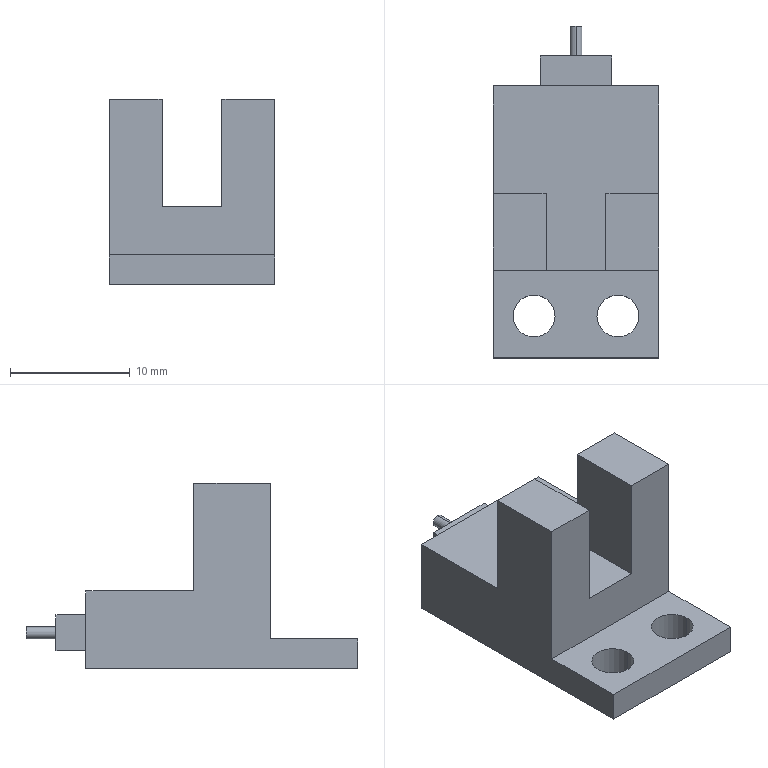Part | SolidWorks | features BaseBody 1 | 1 solid | 26 faces | box 13.8 x 27.7 x 15.5 mm | volume 2139 mm3 | plane 20 | cylinder 6 | commonest cylinder face diameters 3.5 x4 1 x2
STEP:
#1=CARTESIAN_POINT('',(5.25,-14.7,0.));
#2=VERTEX_POINT('',#1);
#3=CARTESIAN_POINT('',(1.75,-14.7,0.));
#4=VERTEX_POINT('',#3);
#5=CARTESIAN_POINT('',(3.5,-14.7,0.));
#6=DIRECTION('',(0.,0.,-1.));
#7=DIRECTION('',(1.,0.,0.));
#8=AXIS2_PLACEMENT_3D('',#5,#6,#7);
#9=CIRCLE('',#8,1.75);
#10=EDGE_CURVE('',#2,#4,#9,.T.);
#11=ORIENTED_EDGE('',*,*,#10,.T.);
#12=CARTESIAN_POINT('',(1.75,-14.7,2.5));
#13=VERTEX_POINT('',#12);
#14=CARTESIAN_POINT('',(1.75,-14.7,2.5));
#15=DIRECTION('',(0.,0.,1.));
#16=VECTOR('',#15,1000.);
#17=LINE('',#14,#16);
#18=EDGE_CURVE('',#4,#13,#17,.T.);
#19=ORIENTED_EDGE('',*,*,#18,.T.);
#20=CARTESIAN_POINT('',(5.25,-14.7,2.5));
#21=VERTEX_POINT('',#20);
#22=CARTESIAN_POINT('',(3.5,-14.7,2.5));
#23=DIRECTION('',(0.,0.,-1.));
#24=DIRECTION('',(1.,0.,0.));
#25=AXIS2_PLACEMENT_3D('',#22,#23,#24);
#26=CIRCLE('',#25,1.75);
#27=EDGE_CURVE('',#21,#13,#26,.T.);
#28=ORIENTED_EDGE('',*,*,#27,.F.);
#29=CARTESIAN_POINT('',(5.25,-14.7,2.5));
#30=DIRECTION('',(0.,0.,1.));
#31=VECTOR('',#30,1000.);
#32=LINE('',#29,#31);
#33=EDGE_CURVE('',#2,#21,#32,.T.);
#34=ORIENTED_EDGE('',*,*,#33,.F.);
#35=EDGE_LOOP('',(#11,#19,#28,#34));
#36=FACE_OUTER_BOUND('',#35,.T.);
#37=CARTESIAN_POINT('',(3.5,-14.7,2.5));
#38=DIRECTION('',(0.,0.,1.));
#39=DIRECTION('',(1.,0.,0.));
#40=AXIS2_PLACEMENT_3D('',#37,#38,#39);
#41=CYLINDRICAL_SURFACE('',#40,1.75);
#42=ADVANCED_FACE('',(#36),#41,.F.);
#43=CARTESIAN_POINT('',(-1.75,-14.7,0.));
#44=VERTEX_POINT('',#43);
#45=CARTESIAN_POINT('',(-5.25,-14.7,0.));
#46=VERTEX_POINT('',#45);
#47=CARTESIAN_POINT('',(-3.5,-14.7,0.));
#48=DIRECTION('',(0.,0.,-1.));
#49=DIRECTION('',(1.,0.,0.));
#50=AXIS2_PLACEMENT_3D('',#47,#48,#49);
#51=CIRCLE('',#50,1.75);
#52=EDGE_CURVE('',#44,#46,#51,.T.);
#53=ORIENTED_EDGE('',*,*,#52,.T.);
#54=CARTESIAN_POINT('',(-5.25,-14.7,2.5));
#55=VERTEX_POINT('',#54);
#56=CARTESIAN_POINT('',(-5.25,-14.7,2.5));
#57=DIRECTION('',(0.,0.,1.));
#58=VECTOR('',#57,1000.);
#59=LINE('',#56,#58);
#60=EDGE_CURVE('',#46,#55,#59,.T.);
#61=ORIENTED_EDGE('',*,*,#60,.T.);
#62=CARTESIAN_POINT('',(-1.75,-14.7,2.5));
#63=VERTEX_POINT('',#62);
#64=CARTESIAN_POINT('',(-3.5,-14.7,2.5));
#65=DIRECTION('',(0.,0.,-1.));
#66=DIRECTION('',(1.,0.,0.));
#67=AXIS2_PLACEMENT_3D('',#64,#65,#66);
#68=CIRCLE('',#67,1.75);
#69=EDGE_CURVE('',#63,#55,#68,.T.);
#70=ORIENTED_EDGE('',*,*,#69,.F.);
#71=CARTESIAN_POINT('',(-1.75,-14.7,2.5));
#72=DIRECTION('',(0.,0.,1.));
#73=VECTOR('',#72,1000.);
#74=LINE('',#71,#73);
#75=EDGE_CURVE('',#44,#63,#74,.T.);
#76=ORIENTED_EDGE('',*,*,#75,.F.);
#77=EDGE_LOOP('',(#53,#61,#70,#76));
#78=FACE_OUTER_BOUND('',#77,.T.);
#79=CARTESIAN_POINT('',(-3.5,-14.7,2.5));
#80=DIRECTION('',(0.,0.,1.));
#81=DIRECTION('',(1.,0.,0.));
#82=AXIS2_PLACEMENT_3D('',#79,#80,#81);
#83=CYLINDRICAL_SURFACE('',#82,1.75);
#84=ADVANCED_FACE('',(#78),#83,.F.);
#85=CARTESIAN_POINT('',(0.,9.5,2.5));
#86=VERTEX_POINT('',#85);
#87=CARTESIAN_POINT('',(0.,9.5,3.5));
#88=VERTEX_POINT('',#87);
#89=CARTESIAN_POINT('',(0.,9.5,3.));
#90=DIRECTION('',(0.,-1.,0.));
#91=DIRECTION('',(0.,0.,-1.));
#92=AXIS2_PLACEMENT_3D('',#89,#90,#91);
#93=CIRCLE('',#92,0.5);
#94=EDGE_CURVE('',#86,#88,#93,.T.);
#95=ORIENTED_EDGE('',*,*,#94,.T.);
#96=CARTESIAN_POINT('',(0.,7.,3.5));
#97=VERTEX_POINT('',#96);
#98=CARTESIAN_POINT('',(0.,9.5,3.5));
#99=DIRECTION('',(0.,-1.,0.));
#100=VECTOR('',#99,1000.);
#101=LINE('',#98,#100);
#102=EDGE_CURVE('',#88,#97,#101,.T.);
#103=ORIENTED_EDGE('',*,*,#102,.T.);
#104=CARTESIAN_POINT('',(0.,7.,2.5));
#105=VERTEX_POINT('',#104);
#106=CARTESIAN_POINT('',(0.,7.,3.));
#107=DIRECTION('',(0.,-1.,0.));
#108=DIRECTION('',(0.,0.,-1.));
#109=AXIS2_PLACEMENT_3D('',#106,#107,#108);
#110=CIRCLE('',#109,0.5);
#111=EDGE_CURVE('',#105,#97,#110,.T.);
#112=ORIENTED_EDGE('',*,*,#111,.F.);
#113=CARTESIAN_POINT('',(0.,9.5,2.5));
#114=DIRECTION('',(0.,-1.,0.));
#115=VECTOR('',#114,1000.);
#116=LINE('',#113,#115);
#117=EDGE_CURVE('',#86,#105,#116,.T.);
#118=ORIENTED_EDGE('',*,*,#117,.F.);
#119=EDGE_LOOP('',(#95,#103,#112,#118));
#120=FACE_OUTER_BOUND('',#119,.T.);
#121=CARTESIAN_POINT('',(0.,9.5,3.));
#122=DIRECTION('',(0.,-1.,0.));
#123=DIRECTION('',(0.,0.,-1.));
#124=AXIS2_PLACEMENT_3D('',#121,#122,#123);
#125=CYLINDRICAL_SURFACE('',#124,0.5);
#126=ADVANCED_FACE('',(#120),#125,.T.);
#127=CARTESIAN_POINT('',(-6.9,-18.2,0.));
#128=VERTEX_POINT('',#127);
#129=CARTESIAN_POINT('',(6.9,-18.2,0.));
#130=VERTEX_POINT('',#129);
#131=CARTESIAN_POINT('',(0.,-18.2,0.));
#132=DIRECTION('',(1.,0.,0.));
#133=VECTOR('',#132,1000.);
#134=LINE('',#131,#133);
#135=EDGE_CURVE('',#128,#130,#134,.T.);
#136=ORIENTED_EDGE('',*,*,#135,.F.);
#137=CARTESIAN_POINT('',(-6.9,4.5,0.));
#138=VERTEX_POINT('',#137);
#139=CARTESIAN_POINT('',(-6.9,0.,0.));
#140=DIRECTION('',(0.,-1.,0.));
#141=VECTOR('',#140,1000.);
#142=LINE('',#139,#141);
#143=EDGE_CURVE('',#138,#128,#142,.T.);
#144=ORIENTED_EDGE('',*,*,#143,.F.);
#145=CARTESIAN_POINT('',(6.9,4.5,0.));
#146=VERTEX_POINT('',#145);
#147=CARTESIAN_POINT('',(0.,4.5,0.));
#148=DIRECTION('',(-1.,0.,0.));
#149=VECTOR('',#148,1000.);
#150=LINE('',#147,#149);
#151=EDGE_CURVE('',#146,#138,#150,.T.);
#152=ORIENTED_EDGE('',*,*,#151,.F.);
#153=CARTESIAN_POINT('',(6.9,0.,0.));
#154=DIRECTION('',(0.,1.,0.));
#155=VECTOR('',#154,1000.);
#156=LINE('',#153,#155);
#157=EDGE_CURVE('',#130,#146,#156,.T.);
#158=ORIENTED_EDGE('',*,*,#157,.F.);
#159=EDGE_LOOP('',(#136,#144,#152,#158));
#160=FACE_OUTER_BOUND('',#159,.T.);
#161=ORIENTED_EDGE('',*,*,#10,.F.);
#162=CARTESIAN_POINT('',(3.5,-14.7,0.));
#163=DIRECTION('',(0.,0.,-1.));
#164=DIRECTION('',(1.,0.,0.));
#165=AXIS2_PLACEMENT_3D('',#162,#163,#164);
#166=CIRCLE('',#165,1.75);
#167=EDGE_CURVE('',#4,#2,#166,.T.);
#168=ORIENTED_EDGE('',*,*,#167,.F.);
#169=EDGE_LOOP('',(#161,#168));
#170=FACE_BOUND('',#169,.T.);
#171=ORIENTED_EDGE('',*,*,#52,.F.);
#172=CARTESIAN_POINT('',(-3.5,-14.7,0.));
#173=DIRECTION('',(0.,0.,-1.));
#174=DIRECTION('',(1.,0.,0.));
#175=AXIS2_PLACEMENT_3D('',#172,#173,#174);
#176=CIRCLE('',#175,1.75);
#177=EDGE_CURVE('',#46,#44,#176,.T.);
#178=ORIENTED_EDGE('',*,*,#177,.F.);
#179=EDGE_LOOP('',(#171,#178));
#180=FACE_BOUND('',#179,.T.);
#181=CARTESIAN_POINT('',(0.,0.,0.));
#182=DIRECTION('',(0.,0.,1.));
#183=DIRECTION('',(1.,0.,0.));
#184=AXIS2_PLACEMENT_3D('',#181,#182,#183);
#185=PLANE('',#184);
#186=ADVANCED_FACE('',(#160,#170,#180),#185,.F.);
#187=CARTESIAN_POINT('',(6.9,4.5,6.5));
#188=VERTEX_POINT('',#187);
#189=CARTESIAN_POINT('',(6.9,4.5,6.5));
#190=DIRECTION('',(0.,0.,-1.));
#191=VECTOR('',#190,1000.);
#192=LINE('',#189,#191);
#193=EDGE_CURVE('',#188,#146,#192,.T.);
#194=ORIENTED_EDGE('',*,*,#193,.F.);
#195=CARTESIAN_POINT('',(6.9,-4.5,6.5));
#196=VERTEX_POINT('',#195);
#197=CARTESIAN_POINT('',(6.9,4.5,6.5));
#198=DIRECTION('',(0.,1.,0.));
#199=VECTOR('',#198,1000.);
#200=LINE('',#197,#199);
#201=EDGE_CURVE('',#196,#188,#200,.T.);
#202=ORIENTED_EDGE('',*,*,#201,.F.);
#203=CARTESIAN_POINT('',(6.9,-4.5,15.5));
#204=VERTEX_POINT('',#203);
#205=CARTESIAN_POINT('',(6.9,-4.5,6.5));
#206=DIRECTION('',(0.,0.,-1.));
#207=VECTOR('',#206,1000.);
#208=LINE('',#205,#207);
#209=EDGE_CURVE('',#204,#196,#208,.T.);
#210=ORIENTED_EDGE('',*,*,#209,.F.);
#211=CARTESIAN_POINT('',(6.9,-10.9,15.5));
#212=VERTEX_POINT('',#211);
#213=CARTESIAN_POINT('',(6.9,4.5,15.5));
#214=DIRECTION('',(0.,1.,0.));
#215=VECTOR('',#214,1000.);
#216=LINE('',#213,#215);
#217=EDGE_CURVE('',#212,#204,#216,.T.);
#218=ORIENTED_EDGE('',*,*,#217,.F.);
#219=CARTESIAN_POINT('',(6.9,-10.9,2.5));
#220=VERTEX_POINT('',#219);
#221=CARTESIAN_POINT('',(6.9,-10.9,6.5));
#222=DIRECTION('',(0.,0.,1.));
#223=VECTOR('',#222,1000.);
#224=LINE('',#221,#223);
#225=EDGE_CURVE('',#220,#212,#224,.T.);
#226=ORIENTED_EDGE('',*,*,#225,.F.);
#227=CARTESIAN_POINT('',(6.9,-18.2,2.5));
#228=VERTEX_POINT('',#227);
#229=CARTESIAN_POINT('',(6.9,4.5,2.5));
#230=DIRECTION('',(0.,1.,0.));
#231=VECTOR('',#230,1000.);
#232=LINE('',#229,#231);
#233=EDGE_CURVE('',#228,#220,#232,.T.);
#234=ORIENTED_EDGE('',*,*,#233,.F.);
#235=CARTESIAN_POINT('',(6.9,-18.2,6.5));
#236=DIRECTION('',(0.,0.,1.));
#237=VECTOR('',#236,1000.);
#238=LINE('',#235,#237);
#239=EDGE_CURVE('',#130,#228,#238,.T.);
#240=ORIENTED_EDGE('',*,*,#239,.F.);
#241=ORIENTED_EDGE('',*,*,#157,.T.);
#242=EDGE_LOOP('',(#194,#202,#210,#218,#226,#234,#240,#241));
#243=FACE_OUTER_BOUND('',#242,.T.);
#244=CARTESIAN_POINT('',(6.9,4.5,6.5));
#245=DIRECTION('',(-1.,0.,0.));
#246=DIRECTION('',(0.,-1.,0.));
#247=AXIS2_PLACEMENT_3D('',#244,#245,#246);
#248=PLANE('',#247);
#249=ADVANCED_FACE('',(#243),#248,.F.);
#250=ORIENTED_EDGE('',*,*,#135,.T.);
#251=ORIENTED_EDGE('',*,*,#239,.T.);
#252=CARTESIAN_POINT('',(-6.9,-18.2,2.5));
#253=VERTEX_POINT('',#252);
#254=CARTESIAN_POINT('',(0.,-18.2,2.5));
#255=DIRECTION('',(1.,0.,0.));
#256=VECTOR('',#255,1000.);
#257=LINE('',#254,#256);
#258=EDGE_CURVE('',#253,#228,#257,.T.);
#259=ORIENTED_EDGE('',*,*,#258,.F.);
#260=CARTESIAN_POINT('',(-6.9,-18.2,0.));
#261=DIRECTION('',(0.,0.,1.));
#262=VECTOR('',#261,1000.);
#263=LINE('',#260,#262);
#264=EDGE_CURVE('',#128,#253,#263,.T.);
#265=ORIENTED_EDGE('',*,*,#264,.F.);
#266=EDGE_LOOP('',(#250,#251,#259,#265));
#267=FACE_OUTER_BOUND('',#266,.T.);
#268=CARTESIAN_POINT('',(0.,-18.2,0.));
#269=DIRECTION('',(0.,1.,0.));
#270=DIRECTION('',(0.,0.,1.));
#271=AXIS2_PLACEMENT_3D('',#268,#269,#270);
#272=PLANE('',#271);
#273=ADVANCED_FACE('',(#267),#272,.F.);
#274=ORIENTED_EDGE('',*,*,#264,.T.);
#275=CARTESIAN_POINT('',(-6.9,-10.9,2.5));
#276=VERTEX_POINT('',#275);
#277=CARTESIAN_POINT('',(-6.9,4.5,2.5));
#278=DIRECTION('',(0.,-1.,0.));
#279=VECTOR('',#278,1000.);
#280=LINE('',#277,#279);
#281=EDGE_CURVE('',#276,#253,#280,.T.);
#282=ORIENTED_EDGE('',*,*,#281,.F.);
#283=CARTESIAN_POINT('',(-6.9,-10.9,15.5));
#284=VERTEX_POINT('',#283);
#285=CARTESIAN_POINT('',(-6.9,-10.9,6.5));
#286=DIRECTION('',(0.,0.,-1.));
#287=VECTOR('',#286,1000.);
#288=LINE('',#285,#287);
#289=EDGE_CURVE('',#284,#276,#288,.T.);
#290=ORIENTED_EDGE('',*,*,#289,.F.);
#291=CARTESIAN_POINT('',(-6.9,-4.5,15.5));
#292=VERTEX_POINT('',#291);
#293=CARTESIAN_POINT('',(-6.9,4.5,15.5));
#294=DIRECTION('',(0.,-1.,0.));
#295=VECTOR('',#294,1000.);
#296=LINE('',#293,#295);
#297=EDGE_CURVE('',#292,#284,#296,.T.);
#298=ORIENTED_EDGE('',*,*,#297,.F.);
#299=CARTESIAN_POINT('',(-6.9,-4.5,6.5));
#300=VERTEX_POINT('',#299);
#301=CARTESIAN_POINT('',(-6.9,-4.5,6.5));
#302=DIRECTION('',(0.,0.,1.));
#303=VECTOR('',#302,1000.);
#304=LINE('',#301,#303);
#305=EDGE_CURVE('',#300,#292,#304,.T.);
#306=ORIENTED_EDGE('',*,*,#305,.F.);
#307=CARTESIAN_POINT('',(-6.9,4.5,6.5));
#308=VERTEX_POINT('',#307);
#309=CARTESIAN_POINT('',(-6.9,4.5,6.5));
#310=DIRECTION('',(0.,-1.,0.));
#311=VECTOR('',#310,1000.);
#312=LINE('',#309,#311);
#313=EDGE_CURVE('',#308,#300,#312,.T.);
#314=ORIENTED_EDGE('',*,*,#313,.F.);
#315=CARTESIAN_POINT('',(-6.9,4.5,6.5));
#316=DIRECTION('',(0.,0.,1.));
#317=VECTOR('',#316,1000.);
#318=LINE('',#315,#317);
#319=EDGE_CURVE('',#138,#308,#318,.T.);
#320=ORIENTED_EDGE('',*,*,#319,.F.);
#321=ORIENTED_EDGE('',*,*,#143,.T.);
#322=EDGE_LOOP('',(#274,#282,#290,#298,#306,#314,#320,#321));
#323=FACE_OUTER_BOUND('',#322,.T.);
#324=CARTESIAN_POINT('',(-6.9,4.5,6.5));
#325=DIRECTION('',(1.,0.,0.));
#326=DIRECTION('',(0.,1.,0.));
#327=AXIS2_PLACEMENT_3D('',#324,#325,#326);
#328=PLANE('',#327);
#329=ADVANCED_FACE('',(#323),#328,.F.);
#330=CARTESIAN_POINT('',(3.,4.5,1.5));
#331=VERTEX_POINT('',#330);
#332=CARTESIAN_POINT('',(-3.,4.5,1.5));
#333=VERTEX_POINT('',#332);
#334=CARTESIAN_POINT('',(-6.9,4.5,1.5));
#335=DIRECTION('',(-1.,0.,0.));
#336=VECTOR('',#335,1000.);
#337=LINE('',#334,#336);
#338=EDGE_CURVE('',#331,#333,#337,.T.);
#339=ORIENTED_EDGE('',*,*,#338,.F.);
#340=CARTESIAN_POINT('',(3.,4.5,4.5));
#341=VERTEX_POINT('',#340);
#342=CARTESIAN_POINT('',(3.,4.5,6.5));
#343=DIRECTION('',(0.,0.,-1.));
#344=VECTOR('',#343,1000.);
#345=LINE('',#342,#344);
#346=EDGE_CURVE('',#341,#331,#345,.T.);
#347=ORIENTED_EDGE('',*,*,#346,.F.);
#348=CARTESIAN_POINT('',(-3.,4.5,4.5));
#349=VERTEX_POINT('',#348);
#350=CARTESIAN_POINT('',(-6.9,4.5,4.5));
#351=DIRECTION('',(1.,0.,0.));
#352=VECTOR('',#351,1000.);
#353=LINE('',#350,#352);
#354=EDGE_CURVE('',#349,#341,#353,.T.);
#355=ORIENTED_EDGE('',*,*,#354,.F.);
#356=CARTESIAN_POINT('',(-3.,4.5,6.5));
#357=DIRECTION('',(0.,0.,1.));
#358=VECTOR('',#357,1000.);
#359=LINE('',#356,#358);
#360=EDGE_CURVE('',#333,#349,#359,.T.);
#361=ORIENTED_EDGE('',*,*,#360,.F.);
#362=EDGE_LOOP('',(#339,#347,#355,#361));
#363=FACE_BOUND('',#362,.T.);
#364=ORIENTED_EDGE('',*,*,#319,.T.);
#365=CARTESIAN_POINT('',(-6.9,4.5,6.5));
#366=DIRECTION('',(-1.,0.,0.));
#367=VECTOR('',#366,1000.);
#368=LINE('',#365,#367);
#369=EDGE_CURVE('',#188,#308,#368,.T.);
#370=ORIENTED_EDGE('',*,*,#369,.F.);
#371=ORIENTED_EDGE('',*,*,#193,.T.);
#372=ORIENTED_EDGE('',*,*,#151,.T.);
#373=EDGE_LOOP('',(#364,#370,#371,#372));
#374=FACE_OUTER_BOUND('',#373,.T.);
#375=CARTESIAN_POINT('',(-6.9,4.5,6.5));
#376=DIRECTION('',(0.,-1.,0.));
#377=DIRECTION('',(0.,0.,-1.));
#378=AXIS2_PLACEMENT_3D('',#375,#376,#377);
#379=PLANE('',#378);
#380=ADVANCED_FACE('',(#363,#374),#379,.F.);
#381=ORIENTED_EDGE('',*,*,#18,.F.);
#382=ORIENTED_EDGE('',*,*,#167,.T.);
#383=ORIENTED_EDGE('',*,*,#33,.T.);
#384=CARTESIAN_POINT('',(3.5,-14.7,2.5));
#385=DIRECTION('',(0.,0.,-1.));
#386=DIRECTION('',(1.,0.,0.));
#387=AXIS2_PLACEMENT_3D('',#384,#385,#386);
#388=CIRCLE('',#387,1.75);
#389=EDGE_CURVE('',#13,#21,#388,.T.);
#390=ORIENTED_EDGE('',*,*,#389,.F.);
#391=EDGE_LOOP('',(#381,#382,#383,#390));
#392=FACE_OUTER_BOUND('',#391,.T.);
#393=CARTESIAN_POINT('',(3.5,-14.7,2.5));
#394=DIRECTION('',(0.,0.,1.));
#395=DIRECTION('',(1.,0.,0.));
#396=AXIS2_PLACEMENT_3D('',#393,#394,#395);
#397=CYLINDRICAL_SURFACE('',#396,1.75);
#398=ADVANCED_FACE('',(#392),#397,.F.);
#399=ORIENTED_EDGE('',*,*,#60,.F.);
#400=ORIENTED_EDGE('',*,*,#177,.T.);
#401=ORIENTED_EDGE('',*,*,#75,.T.);
#402=CARTESIAN_POINT('',(-3.5,-14.7,2.5));
#403=DIRECTION('',(0.,0.,-1.));
#404=DIRECTION('',(1.,0.,0.));
#405=AXIS2_PLACEMENT_3D('',#402,#403,#404);
#406=CIRCLE('',#405,1.75);
#407=EDGE_CURVE('',#55,#63,#406,.T.);
#408=ORIENTED_EDGE('',*,*,#407,.F.);
#409=EDGE_LOOP('',(#399,#400,#401,#408));
#410=FACE_OUTER_BOUND('',#409,.T.);
#411=CARTESIAN_POINT('',(-3.5,-14.7,2.5));
#412=DIRECTION('',(0.,0.,1.));
#413=DIRECTION('',(1.,0.,0.));
#414=AXIS2_PLACEMENT_3D('',#411,#412,#413);
#415=CYLINDRICAL_SURFACE('',#414,1.75);
#416=ADVANCED_FACE('',(#410),#415,.F.);
#417=ORIENTED_EDGE('',*,*,#369,.T.);
#418=ORIENTED_EDGE('',*,*,#313,.T.);
#419=CARTESIAN_POINT('',(-2.5,-4.5,6.5));
#420=VERTEX_POINT('',#419);
#421=CARTESIAN_POINT('',(0.,-4.5,6.5));
#422=DIRECTION('',(1.,0.,0.));
#423=VECTOR('',#422,1000.);
#424=LINE('',#421,#423);
#425=EDGE_CURVE('',#300,#420,#424,.T.);
#426=ORIENTED_EDGE('',*,*,#425,.T.);
#427=CARTESIAN_POINT('',(-2.5,-10.9,6.5));
#428=VERTEX_POINT('',#427);
#429=CARTESIAN_POINT('',(-2.5,0.,6.5));
#430=DIRECTION('',(0.,-1.,0.));
#431=VECTOR('',#430,1000.);
#432=LINE('',#429,#431);
#433=EDGE_CURVE('',#420,#428,#432,.T.);
#434=ORIENTED_EDGE('',*,*,#433,.T.);
#435=CARTESIAN_POINT('',(2.5,-10.9,6.5));
#436=VERTEX_POINT('',#435);
#437=CARTESIAN_POINT('',(0.,-10.9,6.5));
#438=DIRECTION('',(1.,0.,0.));
#439=VECTOR('',#438,1000.);
#440=LINE('',#437,#439);
#441=EDGE_CURVE('',#428,#436,#440,.T.);
#442=ORIENTED_EDGE('',*,*,#441,.T.);
#443=CARTESIAN_POINT('',(2.5,-4.5,6.5));
#444=VERTEX_POINT('',#443);
#445=CARTESIAN_POINT('',(2.5,0.,6.5));
#446=DIRECTION('',(0.,1.,0.));
#447=VECTOR('',#446,1000.);
#448=LINE('',#445,#447);
#449=EDGE_CURVE('',#436,#444,#448,.T.);
#450=ORIENTED_EDGE('',*,*,#449,.T.);
#451=CARTESIAN_POINT('',(0.,-4.5,6.5));
#452=DIRECTION('',(1.,0.,0.));
#453=VECTOR('',#452,1000.);
#454=LINE('',#451,#453);
#455=EDGE_CURVE('',#444,#196,#454,.T.);
#456=ORIENTED_EDGE('',*,*,#455,.T.);
#457=ORIENTED_EDGE('',*,*,#201,.T.);
#458=EDGE_LOOP('',(#417,#418,#426,#434,#442,#450,#456,#457));
#459=FACE_OUTER_BOUND('',#458,.T.);
#460=CARTESIAN_POINT('',(0.,0.,6.5));
#461=DIRECTION('',(0.,0.,1.));
#462=DIRECTION('',(1.,0.,0.));
#463=AXIS2_PLACEMENT_3D('',#460,#461,#462);
#464=PLANE('',#463);
#465=ADVANCED_FACE('',(#459),#464,.T.);
#466=CARTESIAN_POINT('',(2.5,-4.5,15.5));
#467=VERTEX_POINT('',#466);
#468=CARTESIAN_POINT('',(2.5,-4.5,0.));
#469=DIRECTION('',(0.,0.,-1.));
#470=VECTOR('',#469,1000.);
#471=LINE('',#468,#470);
#472=EDGE_CURVE('',#467,#444,#471,.T.);
#473=ORIENTED_EDGE('',*,*,#472,.F.);
#474=CARTESIAN_POINT('',(0.,-4.5,15.5));
#475=DIRECTION('',(-1.,0.,0.));
#476=VECTOR('',#475,1000.);
#477=LINE('',#474,#476);
#478=EDGE_CURVE('',#204,#467,#477,.T.);
#479=ORIENTED_EDGE('',*,*,#478,.F.);
#480=ORIENTED_EDGE('',*,*,#209,.T.);
#481=ORIENTED_EDGE('',*,*,#455,.F.);
#482=EDGE_LOOP('',(#473,#479,#480,#481));
#483=FACE_OUTER_BOUND('',#482,.T.);
#484=CARTESIAN_POINT('',(0.,-4.5,0.));
#485=DIRECTION('',(0.,-1.,0.));
#486=DIRECTION('',(0.,0.,-1.));
#487=AXIS2_PLACEMENT_3D('',#484,#485,#486);
#488=PLANE('',#487);
#489=ADVANCED_FACE('',(#483),#488,.F.);
#490=CARTESIAN_POINT('',(2.5,-10.9,15.5));
#491=VERTEX_POINT('',#490);
#492=CARTESIAN_POINT('',(2.5,-10.9,15.5));
#493=DIRECTION('',(0.,1.,0.));
#494=VECTOR('',#493,1000.);
#495=LINE('',#492,#494);
#496=EDGE_CURVE('',#491,#467,#495,.T.);
#497=ORIENTED_EDGE('',*,*,#496,.F.);
#498=CARTESIAN_POINT('',(6.9,-10.9,15.5));
#499=DIRECTION('',(-1.,0.,0.));
#500=VECTOR('',#499,1000.);
#501=LINE('',#498,#500);
#502=EDGE_CURVE('',#212,#491,#501,.T.);
#503=ORIENTED_EDGE('',*,*,#502,.F.);
#504=ORIENTED_EDGE('',*,*,#217,.T.);
#505=ORIENTED_EDGE('',*,*,#478,.T.);
#506=EDGE_LOOP('',(#497,#503,#504,#505));
#507=FACE_OUTER_BOUND('',#506,.T.);
#508=CARTESIAN_POINT('',(6.9,-10.9,15.5));
#509=DIRECTION('',(0.,0.,-1.));
#510=DIRECTION('',(-1.,0.,0.));
#511=AXIS2_PLACEMENT_3D('',#508,#509,#510);
#512=PLANE('',#511);
#513=ADVANCED_FACE('',(#507),#512,.F.);
#514=CARTESIAN_POINT('',(-2.5,-10.9,15.5));
#515=VERTEX_POINT('',#514);
#516=CARTESIAN_POINT('',(0.,-10.9,15.5));
#517=DIRECTION('',(-1.,0.,0.));
#518=VECTOR('',#517,1000.);
#519=LINE('',#516,#518);
#520=EDGE_CURVE('',#515,#284,#519,.T.);
#521=ORIENTED_EDGE('',*,*,#520,.T.);
#522=ORIENTED_EDGE('',*,*,#289,.T.);
#523=CARTESIAN_POINT('',(0.,-10.9,2.5));
#524=DIRECTION('',(1.,0.,0.));
#525=VECTOR('',#524,1000.);
#526=LINE('',#523,#525);
#527=EDGE_CURVE('',#276,#220,#526,.T.);
#528=ORIENTED_EDGE('',*,*,#527,.T.);
#529=ORIENTED_EDGE('',*,*,#225,.T.);
#530=ORIENTED_EDGE('',*,*,#502,.T.);
#531=CARTESIAN_POINT('',(2.5,-10.9,0.));
#532=DIRECTION('',(0.,0.,-1.));
#533=VECTOR('',#532,1000.);
#534=LINE('',#531,#533);
#535=EDGE_CURVE('',#491,#436,#534,.T.);
#536=ORIENTED_EDGE('',*,*,#535,.T.);
#537=ORIENTED_EDGE('',*,*,#441,.F.);
#538=CARTESIAN_POINT('',(-2.5,-10.9,0.));
#539=DIRECTION('',(0.,0.,1.));
#540=VECTOR('',#539,1000.);
#541=LINE('',#538,#540);
#542=EDGE_CURVE('',#428,#515,#541,.T.);
#543=ORIENTED_EDGE('',*,*,#542,.T.);
#544=EDGE_LOOP('',(#521,#522,#528,#529,#530,#536,#537,#543));
#545=FACE_OUTER_BOUND('',#544,.T.);
#546=CARTESIAN_POINT('',(0.,-10.9,0.));
#547=DIRECTION('',(0.,-1.,0.));
#548=DIRECTION('',(0.,0.,-1.));
#549=AXIS2_PLACEMENT_3D('',#546,#547,#548);
#550=PLANE('',#549);
#551=ADVANCED_FACE('',(#545),#550,.T.);
#552=ORIENTED_EDGE('',*,*,#69,.T.);
#553=ORIENTED_EDGE('',*,*,#407,.T.);
#554=EDGE_LOOP('',(#552,#553));
#555=FACE_BOUND('',#554,.T.);
#556=ORIENTED_EDGE('',*,*,#281,.T.);
#557=ORIENTED_EDGE('',*,*,#258,.T.);
#558=ORIENTED_EDGE('',*,*,#233,.T.);
#559=ORIENTED_EDGE('',*,*,#527,.F.);
#560=EDGE_LOOP('',(#556,#557,#558,#559));
#561=FACE_OUTER_BOUND('',#560,.T.);
#562=ORIENTED_EDGE('',*,*,#27,.T.);
#563=ORIENTED_EDGE('',*,*,#389,.T.);
#564=EDGE_LOOP('',(#562,#563));
#565=FACE_BOUND('',#564,.T.);
#566=CARTESIAN_POINT('',(-6.9,-18.2,2.5));
#567=DIRECTION('',(0.,0.,-1.));
#568=DIRECTION('',(-1.,0.,0.));
#569=AXIS2_PLACEMENT_3D('',#566,#567,#568);
#570=PLANE('',#569);
#571=ADVANCED_FACE('',(#555,#561,#565),#570,.F.);
#572=CARTESIAN_POINT('',(-2.5,-4.5,15.5));
#573=VERTEX_POINT('',#572);
#574=CARTESIAN_POINT('',(-2.5,-10.9,15.5));
#575=DIRECTION('',(0.,-1.,0.));
#576=VECTOR('',#575,1000.);
#577=LINE('',#574,#576);
#578=EDGE_CURVE('',#573,#515,#577,.T.);
#579=ORIENTED_EDGE('',*,*,#578,.F.);
#580=CARTESIAN_POINT('',(6.9,-4.5,15.5));
#581=DIRECTION('',(1.,0.,0.));
#582=VECTOR('',#581,1000.);
#583=LINE('',#580,#582);
#584=EDGE_CURVE('',#292,#573,#583,.T.);
#585=ORIENTED_EDGE('',*,*,#584,.F.);
#586=ORIENTED_EDGE('',*,*,#297,.T.);
#587=ORIENTED_EDGE('',*,*,#520,.F.);
#588=EDGE_LOOP('',(#579,#585,#586,#587));
#589=FACE_OUTER_BOUND('',#588,.T.);
#590=CARTESIAN_POINT('',(6.9,-10.9,15.5));
#591=DIRECTION('',(0.,0.,-1.));
#592=DIRECTION('',(-1.,0.,0.));
#593=AXIS2_PLACEMENT_3D('',#590,#591,#592);
#594=PLANE('',#593);
#595=ADVANCED_FACE('',(#589),#594,.F.);
#596=CARTESIAN_POINT('',(-2.5,-4.5,0.));
#597=DIRECTION('',(0.,0.,1.));
#598=VECTOR('',#597,1000.);
#599=LINE('',#596,#598);
#600=EDGE_CURVE('',#420,#573,#599,.T.);
#601=ORIENTED_EDGE('',*,*,#600,.F.);
#602=ORIENTED_EDGE('',*,*,#425,.F.);
#603=ORIENTED_EDGE('',*,*,#305,.T.);
#604=ORIENTED_EDGE('',*,*,#584,.T.);
#605=EDGE_LOOP('',(#601,#602,#603,#604));
#606=FACE_OUTER_BOUND('',#605,.T.);
#607=CARTESIAN_POINT('',(0.,-4.5,0.));
#608=DIRECTION('',(0.,-1.,0.));
#609=DIRECTION('',(0.,0.,-1.));
#610=AXIS2_PLACEMENT_3D('',#607,#608,#609);
#611=PLANE('',#610);
#612=ADVANCED_FACE('',(#606),#611,.F.);
#613=CARTESIAN_POINT('',(-3.,7.,4.5));
#614=VERTEX_POINT('',#613);
#615=CARTESIAN_POINT('',(-3.,7.,4.5));
#616=DIRECTION('',(0.,-1.,0.));
#617=VECTOR('',#616,1000.);
#618=LINE('',#615,#617);
#619=EDGE_CURVE('',#614,#349,#618,.T.);
#620=ORIENTED_EDGE('',*,*,#619,.F.);
#621=CARTESIAN_POINT('',(-3.,7.,1.5));
#622=VERTEX_POINT('',#621);
#623=CARTESIAN_POINT('',(-3.,7.,1.5));
#624=DIRECTION('',(0.,0.,1.));
#625=VECTOR('',#624,1000.);
#626=LINE('',#623,#625);
#627=EDGE_CURVE('',#622,#614,#626,.T.);
#628=ORIENTED_EDGE('',*,*,#627,.F.);
#629=CARTESIAN_POINT('',(-3.,7.,1.5));
#630=DIRECTION('',(0.,1.,0.));
#631=VECTOR('',#630,1000.);
#632=LINE('',#629,#631);
#633=EDGE_CURVE('',#333,#622,#632,.T.);
#634=ORIENTED_EDGE('',*,*,#633,.F.);
#635=ORIENTED_EDGE('',*,*,#360,.T.);
#636=EDGE_LOOP('',(#620,#628,#634,#635));
#637=FACE_OUTER_BOUND('',#636,.T.);
#638=CARTESIAN_POINT('',(-3.,7.,1.5));
#639=DIRECTION('',(1.,0.,0.));
#640=DIRECTION('',(0.,0.,-1.));
#641=AXIS2_PLACEMENT_3D('',#638,#639,#640);
#642=PLANE('',#641);
#643=ADVANCED_FACE('',(#637),#642,.F.);
#644=ORIENTED_EDGE('',*,*,#633,.T.);
#645=CARTESIAN_POINT('',(3.,7.,1.5));
#646=VERTEX_POINT('',#645);
#647=CARTESIAN_POINT('',(-3.,7.,1.5));
#648=DIRECTION('',(-1.,0.,0.));
#649=VECTOR('',#648,1000.);
#650=LINE('',#647,#649);
#651=EDGE_CURVE('',#646,#622,#650,.T.);
#652=ORIENTED_EDGE('',*,*,#651,.F.);
#653=CARTESIAN_POINT('',(3.,7.,1.5));
#654=DIRECTION('',(0.,1.,0.));
#655=VECTOR('',#654,1000.);
#656=LINE('',#653,#655);
#657=EDGE_CURVE('',#331,#646,#656,.T.);
#658=ORIENTED_EDGE('',*,*,#657,.F.);
#659=ORIENTED_EDGE('',*,*,#338,.T.);
#660=EDGE_LOOP('',(#644,#652,#658,#659));
#661=FACE_OUTER_BOUND('',#660,.T.);
#662=CARTESIAN_POINT('',(-3.,7.,1.5));
#663=DIRECTION('',(0.,0.,1.));
#664=DIRECTION('',(1.,0.,0.));
#665=AXIS2_PLACEMENT_3D('',#662,#663,#664);
#666=PLANE('',#665);
#667=ADVANCED_FACE('',(#661),#666,.F.);
#668=ORIENTED_EDGE('',*,*,#657,.T.);
#669=CARTESIAN_POINT('',(3.,7.,4.5));
#670=VERTEX_POINT('',#669);
#671=CARTESIAN_POINT('',(3.,7.,1.5));
#672=DIRECTION('',(0.,0.,-1.));
#673=VECTOR('',#672,1000.);
#674=LINE('',#671,#673);
#675=EDGE_CURVE('',#670,#646,#674,.T.);
#676=ORIENTED_EDGE('',*,*,#675,.F.);
#677=CARTESIAN_POINT('',(3.,7.,4.5));
#678=DIRECTION('',(0.,1.,0.));
#679=VECTOR('',#678,1000.);
#680=LINE('',#677,#679);
#681=EDGE_CURVE('',#341,#670,#680,.T.);
#682=ORIENTED_EDGE('',*,*,#681,.F.);
#683=ORIENTED_EDGE('',*,*,#346,.T.);
#684=EDGE_LOOP('',(#668,#676,#682,#683));
#685=FACE_OUTER_BOUND('',#684,.T.);
#686=CARTESIAN_POINT('',(3.,7.,1.5));
#687=DIRECTION('',(-1.,0.,0.));
#688=DIRECTION('',(0.,0.,1.));
#689=AXIS2_PLACEMENT_3D('',#686,#687,#688);
#690=PLANE('',#689);
#691=ADVANCED_FACE('',(#685),#690,.F.);
#692=ORIENTED_EDGE('',*,*,#681,.T.);
#693=CARTESIAN_POINT('',(-3.,7.,4.5));
#694=DIRECTION('',(1.,0.,0.));
#695=VECTOR('',#694,1000.);
#696=LINE('',#693,#695);
#697=EDGE_CURVE('',#614,#670,#696,.T.);
#698=ORIENTED_EDGE('',*,*,#697,.F.);
#699=ORIENTED_EDGE('',*,*,#619,.T.);
#700=ORIENTED_EDGE('',*,*,#354,.T.);
#701=EDGE_LOOP('',(#692,#698,#699,#700));
#702=FACE_OUTER_BOUND('',#701,.T.);
#703=CARTESIAN_POINT('',(-3.,7.,4.5));
#704=DIRECTION('',(0.,0.,-1.));
#705=DIRECTION('',(-1.,0.,0.));
#706=AXIS2_PLACEMENT_3D('',#703,#704,#705);
#707=PLANE('',#706);
#708=ADVANCED_FACE('',(#702),#707,.F.);
#709=ORIENTED_EDGE('',*,*,#496,.T.);
#710=ORIENTED_EDGE('',*,*,#472,.T.);
#711=ORIENTED_EDGE('',*,*,#449,.F.);
#712=ORIENTED_EDGE('',*,*,#535,.F.);
#713=EDGE_LOOP('',(#709,#710,#711,#712));
#714=FACE_OUTER_BOUND('',#713,.T.);
#715=CARTESIAN_POINT('',(2.5,-3.617,6.5));
#716=DIRECTION('',(1.,0.,0.));
#717=DIRECTION('',(0.,1.,0.));
#718=AXIS2_PLACEMENT_3D('',#715,#716,#717);
#719=PLANE('',#718);
#720=ADVANCED_FACE('',(#714),#719,.F.);
#721=ORIENTED_EDGE('',*,*,#433,.F.);
#722=ORIENTED_EDGE('',*,*,#600,.T.);
#723=ORIENTED_EDGE('',*,*,#578,.T.);
#724=ORIENTED_EDGE('',*,*,#542,.F.);
#725=EDGE_LOOP('',(#721,#722,#723,#724));
#726=FACE_OUTER_BOUND('',#725,.T.);
#727=CARTESIAN_POINT('',(-2.5,-3.617,6.5));
#728=DIRECTION('',(-1.,0.,0.));
#729=DIRECTION('',(0.,-1.,0.));
#730=AXIS2_PLACEMENT_3D('',#727,#728,#729);
#731=PLANE('',#730);
#732=ADVANCED_FACE('',(#726),#731,.F.);
#733=ORIENTED_EDGE('',*,*,#675,.T.);
#734=ORIENTED_EDGE('',*,*,#651,.T.);
#735=ORIENTED_EDGE('',*,*,#627,.T.);
#736=ORIENTED_EDGE('',*,*,#697,.T.);
#737=EDGE_LOOP('',(#733,#734,#735,#736));
#738=FACE_OUTER_BOUND('',#737,.T.);
#739=ORIENTED_EDGE('',*,*,#111,.T.);
#740=CARTESIAN_POINT('',(0.,7.,3.));
#741=DIRECTION('',(0.,-1.,0.));
#742=DIRECTION('',(0.,0.,-1.));
#743=AXIS2_PLACEMENT_3D('',#740,#741,#742);
#744=CIRCLE('',#743,0.5);
#745=EDGE_CURVE('',#97,#105,#744,.T.);
#746=ORIENTED_EDGE('',*,*,#745,.T.);
#747=EDGE_LOOP('',(#739,#746));
#748=FACE_BOUND('',#747,.T.);
#749=CARTESIAN_POINT('',(0.,7.,0.));
#750=DIRECTION('',(0.,1.,0.));
#751=DIRECTION('',(0.,0.,1.));
#752=AXIS2_PLACEMENT_3D('',#749,#750,#751);
#753=PLANE('',#752);
#754=ADVANCED_FACE('',(#738,#748),#753,.T.);
#755=ORIENTED_EDGE('',*,*,#102,.F.);
#756=CARTESIAN_POINT('',(0.,9.5,3.));
#757=DIRECTION('',(0.,-1.,0.));
#758=DIRECTION('',(0.,0.,-1.));
#759=AXIS2_PLACEMENT_3D('',#756,#757,#758);
#760=CIRCLE('',#759,0.5);
#761=EDGE_CURVE('',#88,#86,#760,.T.);
#762=ORIENTED_EDGE('',*,*,#761,.T.);
#763=ORIENTED_EDGE('',*,*,#117,.T.);
#764=ORIENTED_EDGE('',*,*,#745,.F.);
#765=EDGE_LOOP('',(#755,#762,#763,#764));
#766=FACE_OUTER_BOUND('',#765,.T.);
#767=CARTESIAN_POINT('',(0.,9.5,3.));
#768=DIRECTION('',(0.,-1.,0.));
#769=DIRECTION('',(0.,0.,-1.));
#770=AXIS2_PLACEMENT_3D('',#767,#768,#769);
#771=CYLINDRICAL_SURFACE('',#770,0.5);
#772=ADVANCED_FACE('',(#766),#771,.T.);
#773=ORIENTED_EDGE('',*,*,#94,.F.);
#774=ORIENTED_EDGE('',*,*,#761,.F.);
#775=EDGE_LOOP('',(#773,#774));
#776=FACE_OUTER_BOUND('',#775,.T.);
#777=CARTESIAN_POINT('',(0.,9.5,3.));
#778=DIRECTION('',(0.,1.,0.));
#779=DIRECTION('',(0.,0.,1.));
#780=AXIS2_PLACEMENT_3D('',#777,#778,#779);
#781=PLANE('',#780);
#782=ADVANCED_FACE('',(#776),#781,.T.);
#783=CLOSED_SHELL('',(#42,#84,#126,#186,#249,#273,#329,#380,#398,#416,#465,#489,#513,#551,#571,#595,#612,#643,#667,#691,#708,#720,#732,#754,#772,#782));
#784=MANIFOLD_SOLID_BREP('',#783);
#785=CARTESIAN_POINT('',(0.,0.,0.));
#786=DIRECTION('',(0.,0.,1.));
#787=DIRECTION('',(1.,0.,0.));
#788=AXIS2_PLACEMENT_3D('',#785,#786,#787);
#789=(LENGTH_UNIT()NAMED_UNIT(*)SI_UNIT(.MILLI.,.METRE.));
#790=UNCERTAINTY_MEASURE_WITH_UNIT(LENGTH_MEASURE(0.00001),#789,'','');
#791=(NAMED_UNIT(*)PLANE_ANGLE_UNIT()SI_UNIT($,.RADIAN.));
#792=(NAMED_UNIT(*)SI_UNIT($,.STERADIAN.)SOLID_ANGLE_UNIT());
#793=(GEOMETRIC_REPRESENTATION_CONTEXT(3)GLOBAL_UNCERTAINTY_ASSIGNED_CONTEXT((#790))GLOBAL_UNIT_ASSIGNED_CONTEXT((#789,#791,#792))REPRESENTATION_CONTEXT('',''));
#794=ADVANCED_BREP_SHAPE_REPRESENTATION('',(#784,#788),#793);